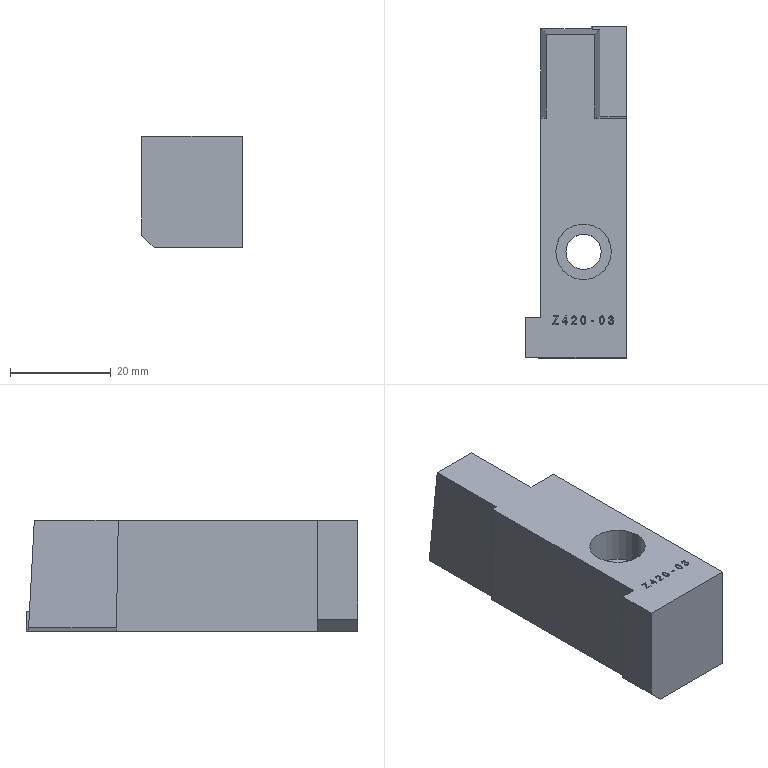Part | Creo | 1 solid | 155 faces | box 20 x 65.745 x 22.097 mm | volume 21449 mm3 | other 93 | plane 56 | cylinder 6 | commonest cylinder face diameters 7 x2 11 x2 1.421 x1 22.406 x1